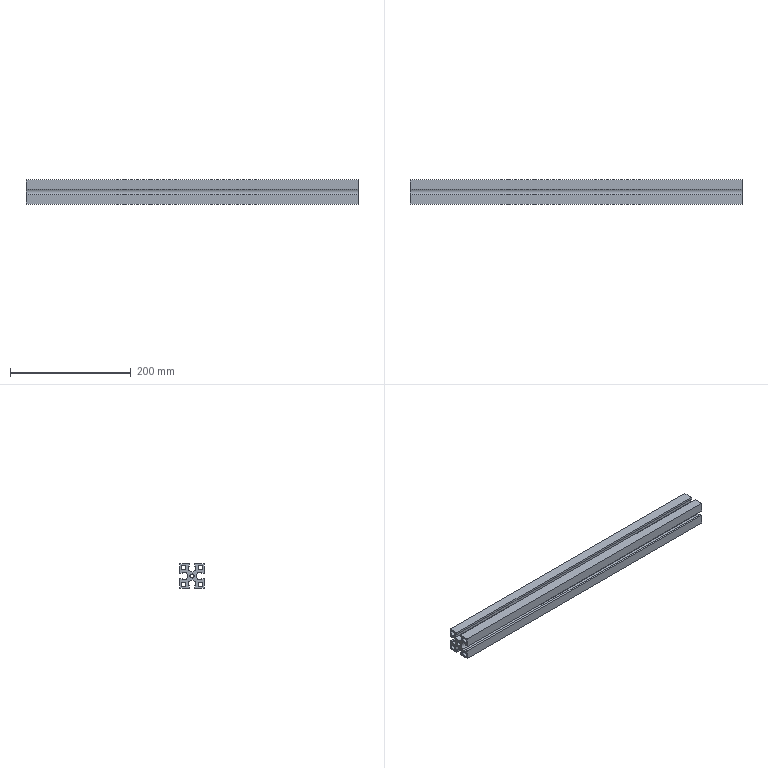Part | NX | 1 solid | 43 faces | box 550 x 40 x 40 mm | volume 437741 mm3 | plane 34 | cylinder 9 | commonest cylinder face diameters 8 x4 20 x4 6.8 x1
STEP:
#1=CARTESIAN_POINT('',(0.,20.,4.25));
#2=VERTEX_POINT('',#1);
#3=CARTESIAN_POINT('',(0.,20.,20.));
#4=VERTEX_POINT('',#3);
#5=CARTESIAN_POINT('',(0.,20.,4.25));
#6=DIRECTION('',(0.,0.,1.));
#7=VECTOR('',#6,1000.);
#8=LINE('',#5,#7);
#9=EDGE_CURVE('',#2,#4,#8,.T.);
#10=ORIENTED_EDGE('',*,*,#9,.T.);
#11=CARTESIAN_POINT('',(550.,20.,20.));
#12=VERTEX_POINT('',#11);
#13=CARTESIAN_POINT('',(550.,20.,20.));
#14=DIRECTION('',(-1.,0.,0.));
#15=VECTOR('',#14,1000.);
#16=LINE('',#13,#15);
#17=EDGE_CURVE('',#12,#4,#16,.T.);
#18=ORIENTED_EDGE('',*,*,#17,.F.);
#19=CARTESIAN_POINT('',(550.,20.,4.25));
#20=VERTEX_POINT('',#19);
#21=CARTESIAN_POINT('',(550.,20.,4.25));
#22=DIRECTION('',(0.,0.,1.));
#23=VECTOR('',#22,1000.);
#24=LINE('',#21,#23);
#25=EDGE_CURVE('',#20,#12,#24,.T.);
#26=ORIENTED_EDGE('',*,*,#25,.F.);
#27=CARTESIAN_POINT('',(550.,20.,4.25));
#28=DIRECTION('',(-1.,0.,0.));
#29=VECTOR('',#28,1000.);
#30=LINE('',#27,#29);
#31=EDGE_CURVE('',#20,#2,#30,.T.);
#32=ORIENTED_EDGE('',*,*,#31,.T.);
#33=EDGE_LOOP('',(#10,#18,#26,#32));
#34=FACE_BOUND('',#33,.T.);
#35=CARTESIAN_POINT('',(550.,20.,4.25));
#36=DIRECTION('',(0.,-1.,0.));
#37=DIRECTION('',(0.,0.,-1.));
#38=AXIS2_PLACEMENT_3D('',#35,#36,#37);
#39=PLANE('',#38);
#40=ADVANCED_FACE('',(#34),#39,.F.);
#41=CARTESIAN_POINT('',(0.,4.25,20.));
#42=VERTEX_POINT('',#41);
#43=CARTESIAN_POINT('',(0.,20.,20.));
#44=DIRECTION('',(0.,-1.,0.));
#45=VECTOR('',#44,1000.);
#46=LINE('',#43,#45);
#47=EDGE_CURVE('',#4,#42,#46,.T.);
#48=ORIENTED_EDGE('',*,*,#47,.T.);
#49=CARTESIAN_POINT('',(550.,4.25,20.));
#50=VERTEX_POINT('',#49);
#51=CARTESIAN_POINT('',(550.,4.25,20.));
#52=DIRECTION('',(-1.,0.,0.));
#53=VECTOR('',#52,1000.);
#54=LINE('',#51,#53);
#55=EDGE_CURVE('',#50,#42,#54,.T.);
#56=ORIENTED_EDGE('',*,*,#55,.F.);
#57=CARTESIAN_POINT('',(550.,20.,20.));
#58=DIRECTION('',(0.,-1.,0.));
#59=VECTOR('',#58,1000.);
#60=LINE('',#57,#59);
#61=EDGE_CURVE('',#12,#50,#60,.T.);
#62=ORIENTED_EDGE('',*,*,#61,.F.);
#63=ORIENTED_EDGE('',*,*,#17,.T.);
#64=EDGE_LOOP('',(#48,#56,#62,#63));
#65=FACE_BOUND('',#64,.T.);
#66=CARTESIAN_POINT('',(550.,20.,20.));
#67=DIRECTION('',(0.,0.,-1.));
#68=DIRECTION('',(0.,1.,0.));
#69=AXIS2_PLACEMENT_3D('',#66,#67,#68);
#70=PLANE('',#69);
#71=ADVANCED_FACE('',(#65),#70,.F.);
#72=CARTESIAN_POINT('',(0.,4.25,16.5));
#73=VERTEX_POINT('',#72);
#74=CARTESIAN_POINT('',(0.,4.25,20.));
#75=DIRECTION('',(0.,0.,-1.));
#76=VECTOR('',#75,1000.);
#77=LINE('',#74,#76);
#78=EDGE_CURVE('',#42,#73,#77,.T.);
#79=ORIENTED_EDGE('',*,*,#78,.T.);
#80=CARTESIAN_POINT('',(550.,4.25,16.5));
#81=VERTEX_POINT('',#80);
#82=CARTESIAN_POINT('',(550.,4.25,16.5));
#83=DIRECTION('',(-1.,0.,0.));
#84=VECTOR('',#83,1000.);
#85=LINE('',#82,#84);
#86=EDGE_CURVE('',#81,#73,#85,.T.);
#87=ORIENTED_EDGE('',*,*,#86,.F.);
#88=CARTESIAN_POINT('',(550.,4.25,20.));
#89=DIRECTION('',(0.,0.,-1.));
#90=VECTOR('',#89,1000.);
#91=LINE('',#88,#90);
#92=EDGE_CURVE('',#50,#81,#91,.T.);
#93=ORIENTED_EDGE('',*,*,#92,.F.);
#94=ORIENTED_EDGE('',*,*,#55,.T.);
#95=EDGE_LOOP('',(#79,#87,#93,#94));
#96=FACE_BOUND('',#95,.T.);
#97=CARTESIAN_POINT('',(550.,4.25,20.));
#98=DIRECTION('',(0.,1.,0.));
#99=DIRECTION('',(0.,0.,1.));
#100=AXIS2_PLACEMENT_3D('',#97,#98,#99);
#101=PLANE('',#100);
#102=ADVANCED_FACE('',(#96),#101,.F.);
#103=CARTESIAN_POINT('',(0.,6.573,16.5));
#104=VERTEX_POINT('',#103);
#105=CARTESIAN_POINT('',(0.,4.25,16.5));
#106=DIRECTION('',(0.,1.,0.));
#107=VECTOR('',#106,1000.);
#108=LINE('',#105,#107);
#109=EDGE_CURVE('',#73,#104,#108,.T.);
#110=ORIENTED_EDGE('',*,*,#109,.T.);
#111=CARTESIAN_POINT('',(550.,6.573,16.5));
#112=VERTEX_POINT('',#111);
#113=CARTESIAN_POINT('',(550.,6.573,16.5));
#114=DIRECTION('',(-1.,0.,0.));
#115=VECTOR('',#114,1000.);
#116=LINE('',#113,#115);
#117=EDGE_CURVE('',#112,#104,#116,.T.);
#118=ORIENTED_EDGE('',*,*,#117,.F.);
#119=CARTESIAN_POINT('',(550.,4.25,16.5));
#120=DIRECTION('',(0.,1.,0.));
#121=VECTOR('',#120,1000.);
#122=LINE('',#119,#121);
#123=EDGE_CURVE('',#81,#112,#122,.T.);
#124=ORIENTED_EDGE('',*,*,#123,.F.);
#125=ORIENTED_EDGE('',*,*,#86,.T.);
#126=EDGE_LOOP('',(#110,#118,#124,#125));
#127=FACE_BOUND('',#126,.T.);
#128=CARTESIAN_POINT('',(550.,4.25,16.5));
#129=DIRECTION('',(0.,0.,1.));
#130=DIRECTION('',(1.,0.,0.));
#131=AXIS2_PLACEMENT_3D('',#128,#129,#130);
#132=PLANE('',#131);
#133=ADVANCED_FACE('',(#127),#132,.F.);
#134=CARTESIAN_POINT('',(0.,6.573,9.673));
#135=VERTEX_POINT('',#134);
#136=CARTESIAN_POINT('',(0.,6.573,16.5));
#137=DIRECTION('',(0.,0.,-1.));
#138=VECTOR('',#137,1000.);
#139=LINE('',#136,#138);
#140=EDGE_CURVE('',#104,#135,#139,.T.);
#141=ORIENTED_EDGE('',*,*,#140,.T.);
#142=CARTESIAN_POINT('',(550.,6.573,9.673));
#143=VERTEX_POINT('',#142);
#144=CARTESIAN_POINT('',(550.,6.573,9.673));
#145=DIRECTION('',(-1.,0.,0.));
#146=VECTOR('',#145,1000.);
#147=LINE('',#144,#146);
#148=EDGE_CURVE('',#143,#135,#147,.T.);
#149=ORIENTED_EDGE('',*,*,#148,.F.);
#150=CARTESIAN_POINT('',(550.,6.573,16.5));
#151=DIRECTION('',(0.,0.,-1.));
#152=VECTOR('',#151,1000.);
#153=LINE('',#150,#152);
#154=EDGE_CURVE('',#112,#143,#153,.T.);
#155=ORIENTED_EDGE('',*,*,#154,.F.);
#156=ORIENTED_EDGE('',*,*,#117,.T.);
#157=EDGE_LOOP('',(#141,#149,#155,#156));
#158=FACE_BOUND('',#157,.T.);
#159=CARTESIAN_POINT('',(550.,6.573,16.5));
#160=DIRECTION('',(0.,1.,0.));
#161=DIRECTION('',(0.,0.,1.));
#162=AXIS2_PLACEMENT_3D('',#159,#160,#161);
#163=PLANE('',#162);
#164=ADVANCED_FACE('',(#158),#163,.F.);
#165=CARTESIAN_POINT('',(0.,-6.573,9.673));
#166=VERTEX_POINT('',#165);
#167=CARTESIAN_POINT('',(0.,0.,17.209));
#168=DIRECTION('',(-1.,0.,0.));
#169=DIRECTION('',(0.,0.,1.));
#170=AXIS2_PLACEMENT_3D('',#167,#168,#169);
#171=CIRCLE('',#170,10.);
#172=EDGE_CURVE('',#135,#166,#171,.T.);
#173=ORIENTED_EDGE('',*,*,#172,.T.);
#174=CARTESIAN_POINT('',(550.,-6.573,9.673));
#175=VERTEX_POINT('',#174);
#176=CARTESIAN_POINT('',(550.,-6.573,9.673));
#177=DIRECTION('',(-1.,0.,0.));
#178=VECTOR('',#177,1000.);
#179=LINE('',#176,#178);
#180=EDGE_CURVE('',#175,#166,#179,.T.);
#181=ORIENTED_EDGE('',*,*,#180,.F.);
#182=CARTESIAN_POINT('',(550.,0.,17.209));
#183=DIRECTION('',(-1.,0.,0.));
#184=DIRECTION('',(0.,0.,1.));
#185=AXIS2_PLACEMENT_3D('',#182,#183,#184);
#186=CIRCLE('',#185,10.);
#187=EDGE_CURVE('',#143,#175,#186,.T.);
#188=ORIENTED_EDGE('',*,*,#187,.F.);
#189=ORIENTED_EDGE('',*,*,#148,.T.);
#190=EDGE_LOOP('',(#173,#181,#188,#189));
#191=FACE_BOUND('',#190,.T.);
#192=CARTESIAN_POINT('',(550.,0.,17.209));
#193=DIRECTION('',(-1.,0.,0.));
#194=DIRECTION('',(0.,0.,1.));
#195=AXIS2_PLACEMENT_3D('',#192,#193,#194);
#196=CYLINDRICAL_SURFACE('',#195,10.);
#197=ADVANCED_FACE('',(#191),#196,.F.);
#198=CARTESIAN_POINT('',(0.,-6.573,16.5));
#199=VERTEX_POINT('',#198);
#200=CARTESIAN_POINT('',(0.,-6.573,9.673));
#201=DIRECTION('',(0.,0.,1.));
#202=VECTOR('',#201,1000.);
#203=LINE('',#200,#202);
#204=EDGE_CURVE('',#166,#199,#203,.T.);
#205=ORIENTED_EDGE('',*,*,#204,.T.);
#206=CARTESIAN_POINT('',(550.,-6.573,16.5));
#207=VERTEX_POINT('',#206);
#208=CARTESIAN_POINT('',(550.,-6.573,16.5));
#209=DIRECTION('',(-1.,0.,0.));
#210=VECTOR('',#209,1000.);
#211=LINE('',#208,#210);
#212=EDGE_CURVE('',#207,#199,#211,.T.);
#213=ORIENTED_EDGE('',*,*,#212,.F.);
#214=CARTESIAN_POINT('',(550.,-6.573,9.673));
#215=DIRECTION('',(0.,0.,1.));
#216=VECTOR('',#215,1000.);
#217=LINE('',#214,#216);
#218=EDGE_CURVE('',#175,#207,#217,.T.);
#219=ORIENTED_EDGE('',*,*,#218,.F.);
#220=ORIENTED_EDGE('',*,*,#180,.T.);
#221=EDGE_LOOP('',(#205,#213,#219,#220));
#222=FACE_BOUND('',#221,.T.);
#223=CARTESIAN_POINT('',(550.,-6.573,9.673));
#224=DIRECTION('',(0.,-1.,0.));
#225=DIRECTION('',(0.,0.,-1.));
#226=AXIS2_PLACEMENT_3D('',#223,#224,#225);
#227=PLANE('',#226);
#228=ADVANCED_FACE('',(#222),#227,.F.);
#229=CARTESIAN_POINT('',(0.,-4.25,16.5));
#230=VERTEX_POINT('',#229);
#231=CARTESIAN_POINT('',(0.,-6.573,16.5));
#232=DIRECTION('',(0.,1.,0.));
#233=VECTOR('',#232,1000.);
#234=LINE('',#231,#233);
#235=EDGE_CURVE('',#199,#230,#234,.T.);
#236=ORIENTED_EDGE('',*,*,#235,.T.);
#237=CARTESIAN_POINT('',(550.,-4.25,16.5));
#238=VERTEX_POINT('',#237);
#239=CARTESIAN_POINT('',(550.,-4.25,16.5));
#240=DIRECTION('',(-1.,0.,0.));
#241=VECTOR('',#240,1000.);
#242=LINE('',#239,#241);
#243=EDGE_CURVE('',#238,#230,#242,.T.);
#244=ORIENTED_EDGE('',*,*,#243,.F.);
#245=CARTESIAN_POINT('',(550.,-6.573,16.5));
#246=DIRECTION('',(0.,1.,0.));
#247=VECTOR('',#246,1000.);
#248=LINE('',#245,#247);
#249=EDGE_CURVE('',#207,#238,#248,.T.);
#250=ORIENTED_EDGE('',*,*,#249,.F.);
#251=ORIENTED_EDGE('',*,*,#212,.T.);
#252=EDGE_LOOP('',(#236,#244,#250,#251));
#253=FACE_BOUND('',#252,.T.);
#254=CARTESIAN_POINT('',(550.,-6.573,16.5));
#255=DIRECTION('',(0.,0.,1.));
#256=DIRECTION('',(1.,0.,0.));
#257=AXIS2_PLACEMENT_3D('',#254,#255,#256);
#258=PLANE('',#257);
#259=ADVANCED_FACE('',(#253),#258,.F.);
#260=CARTESIAN_POINT('',(0.,-4.25,20.));
#261=VERTEX_POINT('',#260);
#262=CARTESIAN_POINT('',(0.,-4.25,16.5));
#263=DIRECTION('',(0.,0.,1.));
#264=VECTOR('',#263,1000.);
#265=LINE('',#262,#264);
#266=EDGE_CURVE('',#230,#261,#265,.T.);
#267=ORIENTED_EDGE('',*,*,#266,.T.);
#268=CARTESIAN_POINT('',(550.,-4.25,20.));
#269=VERTEX_POINT('',#268);
#270=CARTESIAN_POINT('',(550.,-4.25,20.));
#271=DIRECTION('',(-1.,0.,0.));
#272=VECTOR('',#271,1000.);
#273=LINE('',#270,#272);
#274=EDGE_CURVE('',#269,#261,#273,.T.);
#275=ORIENTED_EDGE('',*,*,#274,.F.);
#276=CARTESIAN_POINT('',(550.,-4.25,16.5));
#277=DIRECTION('',(0.,0.,1.));
#278=VECTOR('',#277,1000.);
#279=LINE('',#276,#278);
#280=EDGE_CURVE('',#238,#269,#279,.T.);
#281=ORIENTED_EDGE('',*,*,#280,.F.);
#282=ORIENTED_EDGE('',*,*,#243,.T.);
#283=EDGE_LOOP('',(#267,#275,#281,#282));
#284=FACE_BOUND('',#283,.T.);
#285=CARTESIAN_POINT('',(550.,-4.25,16.5));
#286=DIRECTION('',(0.,-1.,0.));
#287=DIRECTION('',(0.,0.,-1.));
#288=AXIS2_PLACEMENT_3D('',#285,#286,#287);
#289=PLANE('',#288);
#290=ADVANCED_FACE('',(#284),#289,.F.);
#291=CARTESIAN_POINT('',(0.,-20.,20.));
#292=VERTEX_POINT('',#291);
#293=CARTESIAN_POINT('',(0.,-4.25,20.));
#294=DIRECTION('',(0.,-1.,0.));
#295=VECTOR('',#294,1000.);
#296=LINE('',#293,#295);
#297=EDGE_CURVE('',#261,#292,#296,.T.);
#298=ORIENTED_EDGE('',*,*,#297,.T.);
#299=CARTESIAN_POINT('',(550.,-20.,20.));
#300=VERTEX_POINT('',#299);
#301=CARTESIAN_POINT('',(550.,-20.,20.));
#302=DIRECTION('',(-1.,0.,0.));
#303=VECTOR('',#302,1000.);
#304=LINE('',#301,#303);
#305=EDGE_CURVE('',#300,#292,#304,.T.);
#306=ORIENTED_EDGE('',*,*,#305,.F.);
#307=CARTESIAN_POINT('',(550.,-4.25,20.));
#308=DIRECTION('',(0.,-1.,0.));
#309=VECTOR('',#308,1000.);
#310=LINE('',#307,#309);
#311=EDGE_CURVE('',#269,#300,#310,.T.);
#312=ORIENTED_EDGE('',*,*,#311,.F.);
#313=ORIENTED_EDGE('',*,*,#274,.T.);
#314=EDGE_LOOP('',(#298,#306,#312,#313));
#315=FACE_BOUND('',#314,.T.);
#316=CARTESIAN_POINT('',(550.,-4.25,20.));
#317=DIRECTION('',(0.,0.,-1.));
#318=DIRECTION('',(0.,1.,0.));
#319=AXIS2_PLACEMENT_3D('',#316,#317,#318);
#320=PLANE('',#319);
#321=ADVANCED_FACE('',(#315),#320,.F.);
#322=CARTESIAN_POINT('',(0.,-20.,4.25));
#323=VERTEX_POINT('',#322);
#324=CARTESIAN_POINT('',(0.,-20.,20.));
#325=DIRECTION('',(0.,0.,-1.));
#326=VECTOR('',#325,1000.);
#327=LINE('',#324,#326);
#328=EDGE_CURVE('',#292,#323,#327,.T.);
#329=ORIENTED_EDGE('',*,*,#328,.T.);
#330=CARTESIAN_POINT('',(550.,-20.,4.25));
#331=VERTEX_POINT('',#330);
#332=CARTESIAN_POINT('',(550.,-20.,4.25));
#333=DIRECTION('',(-1.,0.,0.));
#334=VECTOR('',#333,1000.);
#335=LINE('',#332,#334);
#336=EDGE_CURVE('',#331,#323,#335,.T.);
#337=ORIENTED_EDGE('',*,*,#336,.F.);
#338=CARTESIAN_POINT('',(550.,-20.,20.));
#339=DIRECTION('',(0.,0.,-1.));
#340=VECTOR('',#339,1000.);
#341=LINE('',#338,#340);
#342=EDGE_CURVE('',#300,#331,#341,.T.);
#343=ORIENTED_EDGE('',*,*,#342,.F.);
#344=ORIENTED_EDGE('',*,*,#305,.T.);
#345=EDGE_LOOP('',(#329,#337,#343,#344));
#346=FACE_BOUND('',#345,.T.);
#347=CARTESIAN_POINT('',(550.,-20.,20.));
#348=DIRECTION('',(0.,1.,0.));
#349=DIRECTION('',(0.,0.,1.));
#350=AXIS2_PLACEMENT_3D('',#347,#348,#349);
#351=PLANE('',#350);
#352=ADVANCED_FACE('',(#346),#351,.F.);
#353=CARTESIAN_POINT('',(0.,-16.5,4.25));
#354=VERTEX_POINT('',#353);
#355=CARTESIAN_POINT('',(0.,-20.,4.25));
#356=DIRECTION('',(0.,1.,0.));
#357=VECTOR('',#356,1000.);
#358=LINE('',#355,#357);
#359=EDGE_CURVE('',#323,#354,#358,.T.);
#360=ORIENTED_EDGE('',*,*,#359,.T.);
#361=CARTESIAN_POINT('',(550.,-16.5,4.25));
#362=VERTEX_POINT('',#361);
#363=CARTESIAN_POINT('',(550.,-16.5,4.25));
#364=DIRECTION('',(-1.,0.,0.));
#365=VECTOR('',#364,1000.);
#366=LINE('',#363,#365);
#367=EDGE_CURVE('',#362,#354,#366,.T.);
#368=ORIENTED_EDGE('',*,*,#367,.F.);
#369=CARTESIAN_POINT('',(550.,-20.,4.25));
#370=DIRECTION('',(0.,1.,0.));
#371=VECTOR('',#370,1000.);
#372=LINE('',#369,#371);
#373=EDGE_CURVE('',#331,#362,#372,.T.);
#374=ORIENTED_EDGE('',*,*,#373,.F.);
#375=ORIENTED_EDGE('',*,*,#336,.T.);
#376=EDGE_LOOP('',(#360,#368,#374,#375));
#377=FACE_BOUND('',#376,.T.);
#378=CARTESIAN_POINT('',(550.,-20.,4.25));
#379=DIRECTION('',(0.,0.,1.));
#380=DIRECTION('',(0.,-1.,0.));
#381=AXIS2_PLACEMENT_3D('',#378,#379,#380);
#382=PLANE('',#381);
#383=ADVANCED_FACE('',(#377),#382,.F.);
#384=CARTESIAN_POINT('',(0.,-16.5,6.573));
#385=VERTEX_POINT('',#384);
#386=CARTESIAN_POINT('',(0.,-16.5,4.25));
#387=DIRECTION('',(0.,0.,1.));
#388=VECTOR('',#387,1000.);
#389=LINE('',#386,#388);
#390=EDGE_CURVE('',#354,#385,#389,.T.);
#391=ORIENTED_EDGE('',*,*,#390,.T.);
#392=CARTESIAN_POINT('',(550.,-16.5,6.573));
#393=VERTEX_POINT('',#392);
#394=CARTESIAN_POINT('',(550.,-16.5,6.573));
#395=DIRECTION('',(-1.,0.,0.));
#396=VECTOR('',#395,1000.);
#397=LINE('',#394,#396);
#398=EDGE_CURVE('',#393,#385,#397,.T.);
#399=ORIENTED_EDGE('',*,*,#398,.F.);
#400=CARTESIAN_POINT('',(550.,-16.5,4.25));
#401=DIRECTION('',(0.,0.,1.));
#402=VECTOR('',#401,1000.);
#403=LINE('',#400,#402);
#404=EDGE_CURVE('',#362,#393,#403,.T.);
#405=ORIENTED_EDGE('',*,*,#404,.F.);
#406=ORIENTED_EDGE('',*,*,#367,.T.);
#407=EDGE_LOOP('',(#391,#399,#405,#406));
#408=FACE_BOUND('',#407,.T.);
#409=CARTESIAN_POINT('',(550.,-16.5,4.25));
#410=DIRECTION('',(0.,-1.,0.));
#411=DIRECTION('',(0.,0.,-1.));
#412=AXIS2_PLACEMENT_3D('',#409,#410,#411);
#413=PLANE('',#412);
#414=ADVANCED_FACE('',(#408),#413,.F.);
#415=CARTESIAN_POINT('',(0.,-9.673,6.573));
#416=VERTEX_POINT('',#415);
#417=CARTESIAN_POINT('',(0.,-16.5,6.573));
#418=DIRECTION('',(0.,1.,0.));
#419=VECTOR('',#418,1000.);
#420=LINE('',#417,#419);
#421=EDGE_CURVE('',#385,#416,#420,.T.);
#422=ORIENTED_EDGE('',*,*,#421,.T.);
#423=CARTESIAN_POINT('',(550.,-9.673,6.573));
#424=VERTEX_POINT('',#423);
#425=CARTESIAN_POINT('',(550.,-9.673,6.573));
#426=DIRECTION('',(-1.,0.,0.));
#427=VECTOR('',#426,1000.);
#428=LINE('',#425,#427);
#429=EDGE_CURVE('',#424,#416,#428,.T.);
#430=ORIENTED_EDGE('',*,*,#429,.F.);
#431=CARTESIAN_POINT('',(550.,-16.5,6.573));
#432=DIRECTION('',(0.,1.,0.));
#433=VECTOR('',#432,1000.);
#434=LINE('',#431,#433);
#435=EDGE_CURVE('',#393,#424,#434,.T.);
#436=ORIENTED_EDGE('',*,*,#435,.F.);
#437=ORIENTED_EDGE('',*,*,#398,.T.);
#438=EDGE_LOOP('',(#422,#430,#436,#437));
#439=FACE_BOUND('',#438,.T.);
#440=CARTESIAN_POINT('',(550.,-16.5,6.573));
#441=DIRECTION('',(0.,0.,1.));
#442=DIRECTION('',(0.,-1.,0.));
#443=AXIS2_PLACEMENT_3D('',#440,#441,#442);
#444=PLANE('',#443);
#445=ADVANCED_FACE('',(#439),#444,.F.);
#446=CARTESIAN_POINT('',(0.,-9.673,-6.573));
#447=VERTEX_POINT('',#446);
#448=CARTESIAN_POINT('',(0.,-17.209,0.));
#449=DIRECTION('',(-1.,0.,0.));
#450=DIRECTION('',(0.,0.,1.));
#451=AXIS2_PLACEMENT_3D('',#448,#449,#450);
#452=CIRCLE('',#451,10.);
#453=EDGE_CURVE('',#416,#447,#452,.T.);
#454=ORIENTED_EDGE('',*,*,#453,.T.);
#455=CARTESIAN_POINT('',(550.,-9.673,-6.573));
#456=VERTEX_POINT('',#455);
#457=CARTESIAN_POINT('',(550.,-9.673,-6.573));
#458=DIRECTION('',(-1.,0.,0.));
#459=VECTOR('',#458,1000.);
#460=LINE('',#457,#459);
#461=EDGE_CURVE('',#456,#447,#460,.T.);
#462=ORIENTED_EDGE('',*,*,#461,.F.);
#463=CARTESIAN_POINT('',(550.,-17.209,0.));
#464=DIRECTION('',(-1.,0.,0.));
#465=DIRECTION('',(0.,0.,1.));
#466=AXIS2_PLACEMENT_3D('',#463,#464,#465);
#467=CIRCLE('',#466,10.);
#468=EDGE_CURVE('',#424,#456,#467,.T.);
#469=ORIENTED_EDGE('',*,*,#468,.F.);
#470=ORIENTED_EDGE('',*,*,#429,.T.);
#471=EDGE_LOOP('',(#454,#462,#469,#470));
#472=FACE_BOUND('',#471,.T.);
#473=CARTESIAN_POINT('',(550.,-17.209,0.));
#474=DIRECTION('',(-1.,0.,0.));
#475=DIRECTION('',(0.,0.,1.));
#476=AXIS2_PLACEMENT_3D('',#473,#474,#475);
#477=CYLINDRICAL_SURFACE('',#476,10.);
#478=ADVANCED_FACE('',(#472),#477,.F.);
#479=CARTESIAN_POINT('',(0.,-16.5,-6.573));
#480=VERTEX_POINT('',#479);
#481=CARTESIAN_POINT('',(0.,-9.673,-6.573));
#482=DIRECTION('',(0.,-1.,0.));
#483=VECTOR('',#482,1000.);
#484=LINE('',#481,#483);
#485=EDGE_CURVE('',#447,#480,#484,.T.);
#486=ORIENTED_EDGE('',*,*,#485,.T.);
#487=CARTESIAN_POINT('',(550.,-16.5,-6.573));
#488=VERTEX_POINT('',#487);
#489=CARTESIAN_POINT('',(550.,-16.5,-6.573));
#490=DIRECTION('',(-1.,0.,0.));
#491=VECTOR('',#490,1000.);
#492=LINE('',#489,#491);
#493=EDGE_CURVE('',#488,#480,#492,.T.);
#494=ORIENTED_EDGE('',*,*,#493,.F.);
#495=CARTESIAN_POINT('',(550.,-9.673,-6.573));
#496=DIRECTION('',(0.,-1.,0.));
#497=VECTOR('',#496,1000.);
#498=LINE('',#495,#497);
#499=EDGE_CURVE('',#456,#488,#498,.T.);
#500=ORIENTED_EDGE('',*,*,#499,.F.);
#501=ORIENTED_EDGE('',*,*,#461,.T.);
#502=EDGE_LOOP('',(#486,#494,#500,#501));
#503=FACE_BOUND('',#502,.T.);
#504=CARTESIAN_POINT('',(550.,-9.673,-6.573));
#505=DIRECTION('',(0.,0.,-1.));
#506=DIRECTION('',(0.,1.,0.));
#507=AXIS2_PLACEMENT_3D('',#504,#505,#506);
#508=PLANE('',#507);
#509=ADVANCED_FACE('',(#503),#508,.F.);
#510=CARTESIAN_POINT('',(0.,-16.5,-4.25));
#511=VERTEX_POINT('',#510);
#512=CARTESIAN_POINT('',(0.,-16.5,-6.573));
#513=DIRECTION('',(0.,0.,1.));
#514=VECTOR('',#513,1000.);
#515=LINE('',#512,#514);
#516=EDGE_CURVE('',#480,#511,#515,.T.);
#517=ORIENTED_EDGE('',*,*,#516,.T.);
#518=CARTESIAN_POINT('',(550.,-16.5,-4.25));
#519=VERTEX_POINT('',#518);
#520=CARTESIAN_POINT('',(550.,-16.5,-4.25));
#521=DIRECTION('',(-1.,0.,0.));
#522=VECTOR('',#521,1000.);
#523=LINE('',#520,#522);
#524=EDGE_CURVE('',#519,#511,#523,.T.);
#525=ORIENTED_EDGE('',*,*,#524,.F.);
#526=CARTESIAN_POINT('',(550.,-16.5,-6.573));
#527=DIRECTION('',(0.,0.,1.));
#528=VECTOR('',#527,1000.);
#529=LINE('',#526,#528);
#530=EDGE_CURVE('',#488,#519,#529,.T.);
#531=ORIENTED_EDGE('',*,*,#530,.F.);
#532=ORIENTED_EDGE('',*,*,#493,.T.);
#533=EDGE_LOOP('',(#517,#525,#531,#532));
#534=FACE_BOUND('',#533,.T.);
#535=CARTESIAN_POINT('',(550.,-16.5,-6.573));
#536=DIRECTION('',(0.,-1.,0.));
#537=DIRECTION('',(0.,0.,-1.));
#538=AXIS2_PLACEMENT_3D('',#535,#536,#537);
#539=PLANE('',#538);
#540=ADVANCED_FACE('',(#534),#539,.F.);
#541=CARTESIAN_POINT('',(0.,-20.,-4.25));
#542=VERTEX_POINT('',#541);
#543=CARTESIAN_POINT('',(0.,-16.5,-4.25));
#544=DIRECTION('',(0.,-1.,0.));
#545=VECTOR('',#544,1000.);
#546=LINE('',#543,#545);
#547=EDGE_CURVE('',#511,#542,#546,.T.);
#548=ORIENTED_EDGE('',*,*,#547,.T.);
#549=CARTESIAN_POINT('',(550.,-20.,-4.25));
#550=VERTEX_POINT('',#549);
#551=CARTESIAN_POINT('',(550.,-20.,-4.25));
#552=DIRECTION('',(-1.,0.,0.));
#553=VECTOR('',#552,1000.);
#554=LINE('',#551,#553);
#555=EDGE_CURVE('',#550,#542,#554,.T.);
#556=ORIENTED_EDGE('',*,*,#555,.F.);
#557=CARTESIAN_POINT('',(550.,-16.5,-4.25));
#558=DIRECTION('',(0.,-1.,0.));
#559=VECTOR('',#558,1000.);
#560=LINE('',#557,#559);
#561=EDGE_CURVE('',#519,#550,#560,.T.);
#562=ORIENTED_EDGE('',*,*,#561,.F.);
#563=ORIENTED_EDGE('',*,*,#524,.T.);
#564=EDGE_LOOP('',(#548,#556,#562,#563));
#565=FACE_BOUND('',#564,.T.);
#566=CARTESIAN_POINT('',(550.,-16.5,-4.25));
#567=DIRECTION('',(0.,0.,-1.));
#568=DIRECTION('',(0.,1.,0.));
#569=AXIS2_PLACEMENT_3D('',#566,#567,#568);
#570=PLANE('',#569);
#571=ADVANCED_FACE('',(#565),#570,.F.);
#572=CARTESIAN_POINT('',(0.,-20.,-20.));
#573=VERTEX_POINT('',#572);
#574=CARTESIAN_POINT('',(0.,-20.,-4.25));
#575=DIRECTION('',(0.,0.,-1.));
#576=VECTOR('',#575,1000.);
#577=LINE('',#574,#576);
#578=EDGE_CURVE('',#542,#573,#577,.T.);
#579=ORIENTED_EDGE('',*,*,#578,.T.);
#580=CARTESIAN_POINT('',(550.,-20.,-20.));
#581=VERTEX_POINT('',#580);
#582=CARTESIAN_POINT('',(550.,-20.,-20.));
#583=DIRECTION('',(-1.,0.,0.));
#584=VECTOR('',#583,1000.);
#585=LINE('',#582,#584);
#586=EDGE_CURVE('',#581,#573,#585,.T.);
#587=ORIENTED_EDGE('',*,*,#586,.F.);
#588=CARTESIAN_POINT('',(550.,-20.,-4.25));
#589=DIRECTION('',(0.,0.,-1.));
#590=VECTOR('',#589,1000.);
#591=LINE('',#588,#590);
#592=EDGE_CURVE('',#550,#581,#591,.T.);
#593=ORIENTED_EDGE('',*,*,#592,.F.);
#594=ORIENTED_EDGE('',*,*,#555,.T.);
#595=EDGE_LOOP('',(#579,#587,#593,#594));
#596=FACE_BOUND('',#595,.T.);
#597=CARTESIAN_POINT('',(550.,-20.,-4.25));
#598=DIRECTION('',(0.,1.,0.));
#599=DIRECTION('',(0.,0.,1.));
#600=AXIS2_PLACEMENT_3D('',#597,#598,#599);
#601=PLANE('',#600);
#602=ADVANCED_FACE('',(#596),#601,.F.);
#603=CARTESIAN_POINT('',(0.,-4.25,-20.));
#604=VERTEX_POINT('',#603);
#605=CARTESIAN_POINT('',(0.,-20.,-20.));
#606=DIRECTION('',(0.,1.,0.));
#607=VECTOR('',#606,1000.);
#608=LINE('',#605,#607);
#609=EDGE_CURVE('',#573,#604,#608,.T.);
#610=ORIENTED_EDGE('',*,*,#609,.T.);
#611=CARTESIAN_POINT('',(550.,-4.25,-20.));
#612=VERTEX_POINT('',#611);
#613=CARTESIAN_POINT('',(550.,-4.25,-20.));
#614=DIRECTION('',(-1.,0.,0.));
#615=VECTOR('',#614,1000.);
#616=LINE('',#613,#615);
#617=EDGE_CURVE('',#612,#604,#616,.T.);
#618=ORIENTED_EDGE('',*,*,#617,.F.);
#619=CARTESIAN_POINT('',(550.,-20.,-20.));
#620=DIRECTION('',(0.,1.,0.));
#621=VECTOR('',#620,1000.);
#622=LINE('',#619,#621);
#623=EDGE_CURVE('',#581,#612,#622,.T.);
#624=ORIENTED_EDGE('',*,*,#623,.F.);
#625=ORIENTED_EDGE('',*,*,#586,.T.);
#626=EDGE_LOOP('',(#610,#618,#624,#625));
#627=FACE_BOUND('',#626,.T.);
#628=CARTESIAN_POINT('',(550.,-20.,-20.));
#629=DIRECTION('',(0.,0.,1.));
#630=DIRECTION('',(1.,0.,0.));
#631=AXIS2_PLACEMENT_3D('',#628,#629,#630);
#632=PLANE('',#631);
#633=ADVANCED_FACE('',(#627),#632,.F.);
#634=CARTESIAN_POINT('',(0.,-4.25,-16.5));
#635=VERTEX_POINT('',#634);
#636=CARTESIAN_POINT('',(0.,-4.25,-20.));
#637=DIRECTION('',(0.,0.,1.));
#638=VECTOR('',#637,1000.);
#639=LINE('',#636,#638);
#640=EDGE_CURVE('',#604,#635,#639,.T.);
#641=ORIENTED_EDGE('',*,*,#640,.T.);
#642=CARTESIAN_POINT('',(550.,-4.25,-16.5));
#643=VERTEX_POINT('',#642);
#644=CARTESIAN_POINT('',(550.,-4.25,-16.5));
#645=DIRECTION('',(-1.,0.,0.));
#646=VECTOR('',#645,1000.);
#647=LINE('',#644,#646);
#648=EDGE_CURVE('',#643,#635,#647,.T.);
#649=ORIENTED_EDGE('',*,*,#648,.F.);
#650=CARTESIAN_POINT('',(550.,-4.25,-20.));
#651=DIRECTION('',(0.,0.,1.));
#652=VECTOR('',#651,1000.);
#653=LINE('',#650,#652);
#654=EDGE_CURVE('',#612,#643,#653,.T.);
#655=ORIENTED_EDGE('',*,*,#654,.F.);
#656=ORIENTED_EDGE('',*,*,#617,.T.);
#657=EDGE_LOOP('',(#641,#649,#655,#656));
#658=FACE_BOUND('',#657,.T.);
#659=CARTESIAN_POINT('',(550.,-4.25,-20.));
#660=DIRECTION('',(0.,-1.,0.));
#661=DIRECTION('',(0.,0.,-1.));
#662=AXIS2_PLACEMENT_3D('',#659,#660,#661);
#663=PLANE('',#662);
#664=ADVANCED_FACE('',(#658),#663,.F.);
#665=CARTESIAN_POINT('',(0.,-6.573,-16.5));
#666=VERTEX_POINT('',#665);
#667=CARTESIAN_POINT('',(0.,-4.25,-16.5));
#668=DIRECTION('',(0.,-1.,0.));
#669=VECTOR('',#668,1000.);
#670=LINE('',#667,#669);
#671=EDGE_CURVE('',#635,#666,#670,.T.);
#672=ORIENTED_EDGE('',*,*,#671,.T.);
#673=CARTESIAN_POINT('',(550.,-6.573,-16.5));
#674=VERTEX_POINT('',#673);
#675=CARTESIAN_POINT('',(550.,-6.573,-16.5));
#676=DIRECTION('',(-1.,0.,0.));
#677=VECTOR('',#676,1000.);
#678=LINE('',#675,#677);
#679=EDGE_CURVE('',#674,#666,#678,.T.);
#680=ORIENTED_EDGE('',*,*,#679,.F.);
#681=CARTESIAN_POINT('',(550.,-4.25,-16.5));
#682=DIRECTION('',(0.,-1.,0.));
#683=VECTOR('',#682,1000.);
#684=LINE('',#681,#683);
#685=EDGE_CURVE('',#643,#674,#684,.T.);
#686=ORIENTED_EDGE('',*,*,#685,.F.);
#687=ORIENTED_EDGE('',*,*,#648,.T.);
#688=EDGE_LOOP('',(#672,#680,#686,#687));
#689=FACE_BOUND('',#688,.T.);
#690=CARTESIAN_POINT('',(550.,-4.25,-16.5));
#691=DIRECTION('',(0.,0.,-1.));
#692=DIRECTION('',(0.,1.,0.));
#693=AXIS2_PLACEMENT_3D('',#690,#691,#692);
#694=PLANE('',#693);
#695=ADVANCED_FACE('',(#689),#694,.F.);
#696=CARTESIAN_POINT('',(0.,-6.573,-9.673));
#697=VERTEX_POINT('',#696);
#698=CARTESIAN_POINT('',(0.,-6.573,-16.5));
#699=DIRECTION('',(0.,0.,1.));
#700=VECTOR('',#699,1000.);
#701=LINE('',#698,#700);
#702=EDGE_CURVE('',#666,#697,#701,.T.);
#703=ORIENTED_EDGE('',*,*,#702,.T.);
#704=CARTESIAN_POINT('',(550.,-6.573,-9.673));
#705=VERTEX_POINT('',#704);
#706=CARTESIAN_POINT('',(550.,-6.573,-9.673));
#707=DIRECTION('',(-1.,0.,0.));
#708=VECTOR('',#707,1000.);
#709=LINE('',#706,#708);
#710=EDGE_CURVE('',#705,#697,#709,.T.);
#711=ORIENTED_EDGE('',*,*,#710,.F.);
#712=CARTESIAN_POINT('',(550.,-6.573,-16.5));
#713=DIRECTION('',(0.,0.,1.));
#714=VECTOR('',#713,1000.);
#715=LINE('',#712,#714);
#716=EDGE_CURVE('',#674,#705,#715,.T.);
#717=ORIENTED_EDGE('',*,*,#716,.F.);
#718=ORIENTED_EDGE('',*,*,#679,.T.);
#719=EDGE_LOOP('',(#703,#711,#717,#718));
#720=FACE_BOUND('',#719,.T.);
#721=CARTESIAN_POINT('',(550.,-6.573,-16.5));
#722=DIRECTION('',(0.,-1.,0.));
#723=DIRECTION('',(0.,0.,-1.));
#724=AXIS2_PLACEMENT_3D('',#721,#722,#723);
#725=PLANE('',#724);
#726=ADVANCED_FACE('',(#720),#725,.F.);
#727=CARTESIAN_POINT('',(0.,6.573,-9.673));
#728=VERTEX_POINT('',#727);
#729=CARTESIAN_POINT('',(0.,0.,-17.209));
#730=DIRECTION('',(-1.,0.,0.));
#731=DIRECTION('',(0.,0.,1.));
#732=AXIS2_PLACEMENT_3D('',#729,#730,#731);
#733=CIRCLE('',#732,10.);
#734=EDGE_CURVE('',#697,#728,#733,.T.);
#735=ORIENTED_EDGE('',*,*,#734,.T.);
#736=CARTESIAN_POINT('',(550.,6.573,-9.673));
#737=VERTEX_POINT('',#736);
#738=CARTESIAN_POINT('',(550.,6.573,-9.673));
#739=DIRECTION('',(-1.,0.,0.));
#740=VECTOR('',#739,1000.);
#741=LINE('',#738,#740);
#742=EDGE_CURVE('',#737,#728,#741,.T.);
#743=ORIENTED_EDGE('',*,*,#742,.F.);
#744=CARTESIAN_POINT('',(550.,0.,-17.209));
#745=DIRECTION('',(-1.,0.,0.));
#746=DIRECTION('',(0.,0.,1.));
#747=AXIS2_PLACEMENT_3D('',#744,#745,#746);
#748=CIRCLE('',#747,10.);
#749=EDGE_CURVE('',#705,#737,#748,.T.);
#750=ORIENTED_EDGE('',*,*,#749,.F.);
#751=ORIENTED_EDGE('',*,*,#710,.T.);
#752=EDGE_LOOP('',(#735,#743,#750,#751));
#753=FACE_BOUND('',#752,.T.);
#754=CARTESIAN_POINT('',(550.,0.,-17.209));
#755=DIRECTION('',(-1.,0.,0.));
#756=DIRECTION('',(0.,0.,1.));
#757=AXIS2_PLACEMENT_3D('',#754,#755,#756);
#758=CYLINDRICAL_SURFACE('',#757,10.);
#759=ADVANCED_FACE('',(#753),#758,.F.);
#760=CARTESIAN_POINT('',(0.,6.573,-16.5));
#761=VERTEX_POINT('',#760);
#762=CARTESIAN_POINT('',(0.,6.573,-9.673));
#763=DIRECTION('',(0.,0.,-1.));
#764=VECTOR('',#763,1000.);
#765=LINE('',#762,#764);
#766=EDGE_CURVE('',#728,#761,#765,.T.);
#767=ORIENTED_EDGE('',*,*,#766,.T.);
#768=CARTESIAN_POINT('',(550.,6.573,-16.5));
#769=VERTEX_POINT('',#768);
#770=CARTESIAN_POINT('',(550.,6.573,-16.5));
#771=DIRECTION('',(-1.,0.,0.));
#772=VECTOR('',#771,1000.);
#773=LINE('',#770,#772);
#774=EDGE_CURVE('',#769,#761,#773,.T.);
#775=ORIENTED_EDGE('',*,*,#774,.F.);
#776=CARTESIAN_POINT('',(550.,6.573,-9.673));
#777=DIRECTION('',(0.,0.,-1.));
#778=VECTOR('',#777,1000.);
#779=LINE('',#776,#778);
#780=EDGE_CURVE('',#737,#769,#779,.T.);
#781=ORIENTED_EDGE('',*,*,#780,.F.);
#782=ORIENTED_EDGE('',*,*,#742,.T.);
#783=EDGE_LOOP('',(#767,#775,#781,#782));
#784=FACE_BOUND('',#783,.T.);
#785=CARTESIAN_POINT('',(550.,6.573,-9.673));
#786=DIRECTION('',(0.,1.,0.));
#787=DIRECTION('',(0.,0.,1.));
#788=AXIS2_PLACEMENT_3D('',#785,#786,#787);
#789=PLANE('',#788);
#790=ADVANCED_FACE('',(#784),#789,.F.);
#791=CARTESIAN_POINT('',(0.,4.25,-16.5));
#792=VERTEX_POINT('',#791);
#793=CARTESIAN_POINT('',(0.,6.573,-16.5));
#794=DIRECTION('',(0.,-1.,0.));
#795=VECTOR('',#794,1000.);
#796=LINE('',#793,#795);
#797=EDGE_CURVE('',#761,#792,#796,.T.);
#798=ORIENTED_EDGE('',*,*,#797,.T.);
#799=CARTESIAN_POINT('',(550.,4.25,-16.5));
#800=VERTEX_POINT('',#799);
#801=CARTESIAN_POINT('',(550.,4.25,-16.5));
#802=DIRECTION('',(-1.,0.,0.));
#803=VECTOR('',#802,1000.);
#804=LINE('',#801,#803);
#805=EDGE_CURVE('',#800,#792,#804,.T.);
#806=ORIENTED_EDGE('',*,*,#805,.F.);
#807=CARTESIAN_POINT('',(550.,6.573,-16.5));
#808=DIRECTION('',(0.,-1.,0.));
#809=VECTOR('',#808,1000.);
#810=LINE('',#807,#809);
#811=EDGE_CURVE('',#769,#800,#810,.T.);
#812=ORIENTED_EDGE('',*,*,#811,.F.);
#813=ORIENTED_EDGE('',*,*,#774,.T.);
#814=EDGE_LOOP('',(#798,#806,#812,#813));
#815=FACE_BOUND('',#814,.T.);
#816=CARTESIAN_POINT('',(550.,6.573,-16.5));
#817=DIRECTION('',(0.,0.,-1.));
#818=DIRECTION('',(0.,1.,0.));
#819=AXIS2_PLACEMENT_3D('',#816,#817,#818);
#820=PLANE('',#819);
#821=ADVANCED_FACE('',(#815),#820,.F.);
#822=CARTESIAN_POINT('',(0.,4.25,-20.));
#823=VERTEX_POINT('',#822);
#824=CARTESIAN_POINT('',(0.,4.25,-16.5));
#825=DIRECTION('',(0.,0.,-1.));
#826=VECTOR('',#825,1000.);
#827=LINE('',#824,#826);
#828=EDGE_CURVE('',#792,#823,#827,.T.);
#829=ORIENTED_EDGE('',*,*,#828,.T.);
#830=CARTESIAN_POINT('',(550.,4.25,-20.));
#831=VERTEX_POINT('',#830);
#832=CARTESIAN_POINT('',(550.,4.25,-20.));
#833=DIRECTION('',(-1.,0.,0.));
#834=VECTOR('',#833,1000.);
#835=LINE('',#832,#834);
#836=EDGE_CURVE('',#831,#823,#835,.T.);
#837=ORIENTED_EDGE('',*,*,#836,.F.);
#838=CARTESIAN_POINT('',(550.,4.25,-16.5));
#839=DIRECTION('',(0.,0.,-1.));
#840=VECTOR('',#839,1000.);
#841=LINE('',#838,#840);
#842=EDGE_CURVE('',#800,#831,#841,.T.);
#843=ORIENTED_EDGE('',*,*,#842,.F.);
#844=ORIENTED_EDGE('',*,*,#805,.T.);
#845=EDGE_LOOP('',(#829,#837,#843,#844));
#846=FACE_BOUND('',#845,.T.);
#847=CARTESIAN_POINT('',(550.,4.25,-16.5));
#848=DIRECTION('',(0.,1.,0.));
#849=DIRECTION('',(0.,0.,1.));
#850=AXIS2_PLACEMENT_3D('',#847,#848,#849);
#851=PLANE('',#850);
#852=ADVANCED_FACE('',(#846),#851,.F.);
#853=CARTESIAN_POINT('',(0.,20.,-20.));
#854=VERTEX_POINT('',#853);
#855=CARTESIAN_POINT('',(0.,4.25,-20.));
#856=DIRECTION('',(0.,1.,0.));
#857=VECTOR('',#856,1000.);
#858=LINE('',#855,#857);
#859=EDGE_CURVE('',#823,#854,#858,.T.);
#860=ORIENTED_EDGE('',*,*,#859,.T.);
#861=CARTESIAN_POINT('',(550.,20.,-20.));
#862=VERTEX_POINT('',#861);
#863=CARTESIAN_POINT('',(550.,20.,-20.));
#864=DIRECTION('',(-1.,0.,0.));
#865=VECTOR('',#864,1000.);
#866=LINE('',#863,#865);
#867=EDGE_CURVE('',#862,#854,#866,.T.);
#868=ORIENTED_EDGE('',*,*,#867,.F.);
#869=CARTESIAN_POINT('',(550.,4.25,-20.));
#870=DIRECTION('',(0.,1.,0.));
#871=VECTOR('',#870,1000.);
#872=LINE('',#869,#871);
#873=EDGE_CURVE('',#831,#862,#872,.T.);
#874=ORIENTED_EDGE('',*,*,#873,.F.);
#875=ORIENTED_EDGE('',*,*,#836,.T.);
#876=EDGE_LOOP('',(#860,#868,#874,#875));
#877=FACE_BOUND('',#876,.T.);
#878=CARTESIAN_POINT('',(550.,4.25,-20.));
#879=DIRECTION('',(0.,0.,1.));
#880=DIRECTION('',(1.,0.,0.));
#881=AXIS2_PLACEMENT_3D('',#878,#879,#880);
#882=PLANE('',#881);
#883=ADVANCED_FACE('',(#877),#882,.F.);
#884=CARTESIAN_POINT('',(0.,20.,-4.25));
#885=VERTEX_POINT('',#884);
#886=CARTESIAN_POINT('',(0.,20.,-20.));
#887=DIRECTION('',(0.,0.,1.));
#888=VECTOR('',#887,1000.);
#889=LINE('',#886,#888);
#890=EDGE_CURVE('',#854,#885,#889,.T.);
#891=ORIENTED_EDGE('',*,*,#890,.T.);
#892=CARTESIAN_POINT('',(550.,20.,-4.25));
#893=VERTEX_POINT('',#892);
#894=CARTESIAN_POINT('',(550.,20.,-4.25));
#895=DIRECTION('',(-1.,0.,0.));
#896=VECTOR('',#895,1000.);
#897=LINE('',#894,#896);
#898=EDGE_CURVE('',#893,#885,#897,.T.);
#899=ORIENTED_EDGE('',*,*,#898,.F.);
#900=CARTESIAN_POINT('',(550.,20.,-20.));
#901=DIRECTION('',(0.,0.,1.));
#902=VECTOR('',#901,1000.);
#903=LINE('',#900,#902);
#904=EDGE_CURVE('',#862,#893,#903,.T.);
#905=ORIENTED_EDGE('',*,*,#904,.F.);
#906=ORIENTED_EDGE('',*,*,#867,.T.);
#907=EDGE_LOOP('',(#891,#899,#905,#906));
#908=FACE_BOUND('',#907,.T.);
#909=CARTESIAN_POINT('',(550.,20.,-20.));
#910=DIRECTION('',(0.,-1.,0.));
#911=DIRECTION('',(0.,0.,-1.));
#912=AXIS2_PLACEMENT_3D('',#909,#910,#911);
#913=PLANE('',#912);
#914=ADVANCED_FACE('',(#908),#913,.F.);
#915=CARTESIAN_POINT('',(0.,16.5,-4.25));
#916=VERTEX_POINT('',#915);
#917=CARTESIAN_POINT('',(0.,20.,-4.25));
#918=DIRECTION('',(0.,-1.,0.));
#919=VECTOR('',#918,1000.);
#920=LINE('',#917,#919);
#921=EDGE_CURVE('',#885,#916,#920,.T.);
#922=ORIENTED_EDGE('',*,*,#921,.T.);
#923=CARTESIAN_POINT('',(550.,16.5,-4.25));
#924=VERTEX_POINT('',#923);
#925=CARTESIAN_POINT('',(550.,16.5,-4.25));
#926=DIRECTION('',(-1.,0.,0.));
#927=VECTOR('',#926,1000.);
#928=LINE('',#925,#927);
#929=EDGE_CURVE('',#924,#916,#928,.T.);
#930=ORIENTED_EDGE('',*,*,#929,.F.);
#931=CARTESIAN_POINT('',(550.,20.,-4.25));
#932=DIRECTION('',(0.,-1.,0.));
#933=VECTOR('',#932,1000.);
#934=LINE('',#931,#933);
#935=EDGE_CURVE('',#893,#924,#934,.T.);
#936=ORIENTED_EDGE('',*,*,#935,.F.);
#937=ORIENTED_EDGE('',*,*,#898,.T.);
#938=EDGE_LOOP('',(#922,#930,#936,#937));
#939=FACE_BOUND('',#938,.T.);
#940=CARTESIAN_POINT('',(550.,20.,-4.25));
#941=DIRECTION('',(0.,0.,-1.));
#942=DIRECTION('',(-1.,0.,0.));
#943=AXIS2_PLACEMENT_3D('',#940,#941,#942);
#944=PLANE('',#943);
#945=ADVANCED_FACE('',(#939),#944,.F.);
#946=CARTESIAN_POINT('',(0.,16.5,-6.573));
#947=VERTEX_POINT('',#946);
#948=CARTESIAN_POINT('',(0.,16.5,-4.25));
#949=DIRECTION('',(0.,0.,-1.));
#950=VECTOR('',#949,1000.);
#951=LINE('',#948,#950);
#952=EDGE_CURVE('',#916,#947,#951,.T.);
#953=ORIENTED_EDGE('',*,*,#952,.T.);
#954=CARTESIAN_POINT('',(550.,16.5,-6.573));
#955=VERTEX_POINT('',#954);
#956=CARTESIAN_POINT('',(550.,16.5,-6.573));
#957=DIRECTION('',(-1.,0.,0.));
#958=VECTOR('',#957,1000.);
#959=LINE('',#956,#958);
#960=EDGE_CURVE('',#955,#947,#959,.T.);
#961=ORIENTED_EDGE('',*,*,#960,.F.);
#962=CARTESIAN_POINT('',(550.,16.5,-4.25));
#963=DIRECTION('',(0.,0.,-1.));
#964=VECTOR('',#963,1000.);
#965=LINE('',#962,#964);
#966=EDGE_CURVE('',#924,#955,#965,.T.);
#967=ORIENTED_EDGE('',*,*,#966,.F.);
#968=ORIENTED_EDGE('',*,*,#929,.T.);
#969=EDGE_LOOP('',(#953,#961,#967,#968));
#970=FACE_BOUND('',#969,.T.);
#971=CARTESIAN_POINT('',(550.,16.5,-4.25));
#972=DIRECTION('',(0.,1.,0.));
#973=DIRECTION('',(0.,0.,1.));
#974=AXIS2_PLACEMENT_3D('',#971,#972,#973);
#975=PLANE('',#974);
#976=ADVANCED_FACE('',(#970),#975,.F.);
#977=CARTESIAN_POINT('',(0.,9.673,-6.573));
#978=VERTEX_POINT('',#977);
#979=CARTESIAN_POINT('',(0.,16.5,-6.573));
#980=DIRECTION('',(0.,-1.,0.));
#981=VECTOR('',#980,1000.);
#982=LINE('',#979,#981);
#983=EDGE_CURVE('',#947,#978,#982,.T.);
#984=ORIENTED_EDGE('',*,*,#983,.T.);
#985=CARTESIAN_POINT('',(550.,9.673,-6.573));
#986=VERTEX_POINT('',#985);
#987=CARTESIAN_POINT('',(550.,9.673,-6.573));
#988=DIRECTION('',(-1.,0.,0.));
#989=VECTOR('',#988,1000.);
#990=LINE('',#987,#989);
#991=EDGE_CURVE('',#986,#978,#990,.T.);
#992=ORIENTED_EDGE('',*,*,#991,.F.);
#993=CARTESIAN_POINT('',(550.,16.5,-6.573));
#994=DIRECTION('',(0.,-1.,0.));
#995=VECTOR('',#994,1000.);
#996=LINE('',#993,#995);
#997=EDGE_CURVE('',#955,#986,#996,.T.);
#998=ORIENTED_EDGE('',*,*,#997,.F.);
#999=ORIENTED_EDGE('',*,*,#960,.T.);
#1000=EDGE_LOOP('',(#984,#992,#998,#999));
#1001=FACE_BOUND('',#1000,.T.);
#1002=CARTESIAN_POINT('',(550.,16.5,-6.573));
#1003=DIRECTION('',(0.,0.,-1.));
#1004=DIRECTION('',(-1.,0.,0.));
#1005=AXIS2_PLACEMENT_3D('',#1002,#1003,#1004);
#1006=PLANE('',#1005);
#1007=ADVANCED_FACE('',(#1001),#1006,.F.);
#1008=CARTESIAN_POINT('',(0.,9.673,6.573));
#1009=VERTEX_POINT('',#1008);
#1010=CARTESIAN_POINT('',(0.,17.209,0.));
#1011=DIRECTION('',(-1.,0.,0.));
#1012=DIRECTION('',(0.,0.,1.));
#1013=AXIS2_PLACEMENT_3D('',#1010,#1011,#1012);
#1014=CIRCLE('',#1013,10.);
#1015=EDGE_CURVE('',#978,#1009,#1014,.T.);
#1016=ORIENTED_EDGE('',*,*,#1015,.T.);
#1017=CARTESIAN_POINT('',(550.,9.673,6.573));
#1018=VERTEX_POINT('',#1017);
#1019=CARTESIAN_POINT('',(550.,9.673,6.573));
#1020=DIRECTION('',(-1.,0.,0.));
#1021=VECTOR('',#1020,1000.);
#1022=LINE('',#1019,#1021);
#1023=EDGE_CURVE('',#1018,#1009,#1022,.T.);
#1024=ORIENTED_EDGE('',*,*,#1023,.F.);
#1025=CARTESIAN_POINT('',(550.,17.209,0.));
#1026=DIRECTION('',(-1.,0.,0.));
#1027=DIRECTION('',(0.,0.,1.));
#1028=AXIS2_PLACEMENT_3D('',#1025,#1026,#1027);
#1029=CIRCLE('',#1028,10.);
#1030=EDGE_CURVE('',#986,#1018,#1029,.T.);
#1031=ORIENTED_EDGE('',*,*,#1030,.F.);
#1032=ORIENTED_EDGE('',*,*,#991,.T.);
#1033=EDGE_LOOP('',(#1016,#1024,#1031,#1032));
#1034=FACE_BOUND('',#1033,.T.);
#1035=CARTESIAN_POINT('',(550.,17.209,0.));
#1036=DIRECTION('',(-1.,0.,0.));
#1037=DIRECTION('',(0.,0.,1.));
#1038=AXIS2_PLACEMENT_3D('',#1035,#1036,#1037);
#1039=CYLINDRICAL_SURFACE('',#1038,10.);
#1040=ADVANCED_FACE('',(#1034),#1039,.F.);
#1041=CARTESIAN_POINT('',(0.,16.5,6.573));
#1042=VERTEX_POINT('',#1041);
#1043=CARTESIAN_POINT('',(0.,9.673,6.573));
#1044=DIRECTION('',(0.,1.,0.));
#1045=VECTOR('',#1044,1000.);
#1046=LINE('',#1043,#1045);
#1047=EDGE_CURVE('',#1009,#1042,#1046,.T.);
#1048=ORIENTED_EDGE('',*,*,#1047,.T.);
#1049=CARTESIAN_POINT('',(550.,16.5,6.573));
#1050=VERTEX_POINT('',#1049);
#1051=CARTESIAN_POINT('',(550.,16.5,6.573));
#1052=DIRECTION('',(-1.,0.,0.));
#1053=VECTOR('',#1052,1000.);
#1054=LINE('',#1051,#1053);
#1055=EDGE_CURVE('',#1050,#1042,#1054,.T.);
#1056=ORIENTED_EDGE('',*,*,#1055,.F.);
#1057=CARTESIAN_POINT('',(550.,9.673,6.573));
#1058=DIRECTION('',(0.,1.,0.));
#1059=VECTOR('',#1058,1000.);
#1060=LINE('',#1057,#1059);
#1061=EDGE_CURVE('',#1018,#1050,#1060,.T.);
#1062=ORIENTED_EDGE('',*,*,#1061,.F.);
#1063=ORIENTED_EDGE('',*,*,#1023,.T.);
#1064=EDGE_LOOP('',(#1048,#1056,#1062,#1063));
#1065=FACE_BOUND('',#1064,.T.);
#1066=CARTESIAN_POINT('',(550.,9.673,6.573));
#1067=DIRECTION('',(0.,0.,1.));
#1068=DIRECTION('',(1.,0.,0.));
#1069=AXIS2_PLACEMENT_3D('',#1066,#1067,#1068);
#1070=PLANE('',#1069);
#1071=ADVANCED_FACE('',(#1065),#1070,.F.);
#1072=CARTESIAN_POINT('',(0.,16.5,4.25));
#1073=VERTEX_POINT('',#1072);
#1074=CARTESIAN_POINT('',(0.,16.5,6.573));
#1075=DIRECTION('',(0.,0.,-1.));
#1076=VECTOR('',#1075,1000.);
#1077=LINE('',#1074,#1076);
#1078=EDGE_CURVE('',#1042,#1073,#1077,.T.);
#1079=ORIENTED_EDGE('',*,*,#1078,.T.);
#1080=CARTESIAN_POINT('',(550.,16.5,4.25));
#1081=VERTEX_POINT('',#1080);
#1082=CARTESIAN_POINT('',(550.,16.5,4.25));
#1083=DIRECTION('',(-1.,0.,0.));
#1084=VECTOR('',#1083,1000.);
#1085=LINE('',#1082,#1084);
#1086=EDGE_CURVE('',#1081,#1073,#1085,.T.);
#1087=ORIENTED_EDGE('',*,*,#1086,.F.);
#1088=CARTESIAN_POINT('',(550.,16.5,6.573));
#1089=DIRECTION('',(0.,0.,-1.));
#1090=VECTOR('',#1089,1000.);
#1091=LINE('',#1088,#1090);
#1092=EDGE_CURVE('',#1050,#1081,#1091,.T.);
#1093=ORIENTED_EDGE('',*,*,#1092,.F.);
#1094=ORIENTED_EDGE('',*,*,#1055,.T.);
#1095=EDGE_LOOP('',(#1079,#1087,#1093,#1094));
#1096=FACE_BOUND('',#1095,.T.);
#1097=CARTESIAN_POINT('',(550.,16.5,6.573));
#1098=DIRECTION('',(0.,1.,0.));
#1099=DIRECTION('',(0.,0.,1.));
#1100=AXIS2_PLACEMENT_3D('',#1097,#1098,#1099);
#1101=PLANE('',#1100);
#1102=ADVANCED_FACE('',(#1096),#1101,.F.);
#1103=CARTESIAN_POINT('',(550.,14.,-10.));
#1104=VERTEX_POINT('',#1103);
#1105=CARTESIAN_POINT('',(550.,14.,-14.));
#1106=DIRECTION('',(1.,0.,0.));
#1107=DIRECTION('',(0.,0.,1.));
#1108=AXIS2_PLACEMENT_3D('',#1105,#1106,#1107);
#1109=CIRCLE('',#1108,4.);
#1110=EDGE_CURVE('',#1104,#1104,#1109,.T.);
#1111=ORIENTED_EDGE('',*,*,#1110,.T.);
#1112=EDGE_LOOP('',(#1111));
#1113=FACE_BOUND('',#1112,.T.);
#1114=CARTESIAN_POINT('',(0.,14.,-10.));
#1115=VERTEX_POINT('',#1114);
#1116=CARTESIAN_POINT('',(0.,14.,-14.));
#1117=DIRECTION('',(1.,0.,0.));
#1118=DIRECTION('',(0.,0.,1.));
#1119=AXIS2_PLACEMENT_3D('',#1116,#1117,#1118);
#1120=CIRCLE('',#1119,4.);
#1121=EDGE_CURVE('',#1115,#1115,#1120,.T.);
#1122=ORIENTED_EDGE('',*,*,#1121,.F.);
#1123=EDGE_LOOP('',(#1122));
#1124=FACE_BOUND('',#1123,.T.);
#1125=CARTESIAN_POINT('',(550.,14.,-14.));
#1126=DIRECTION('',(-1.,0.,0.));
#1127=DIRECTION('',(0.,0.,1.));
#1128=AXIS2_PLACEMENT_3D('',#1125,#1126,#1127);
#1129=CYLINDRICAL_SURFACE('',#1128,4.);
#1130=ADVANCED_FACE('',(#1113,#1124),#1129,.F.);
#1131=CARTESIAN_POINT('',(550.,-14.,18.));
#1132=VERTEX_POINT('',#1131);
#1133=CARTESIAN_POINT('',(550.,-14.,14.));
#1134=DIRECTION('',(1.,0.,0.));
#1135=DIRECTION('',(0.,0.,1.));
#1136=AXIS2_PLACEMENT_3D('',#1133,#1134,#1135);
#1137=CIRCLE('',#1136,4.);
#1138=EDGE_CURVE('',#1132,#1132,#1137,.T.);
#1139=ORIENTED_EDGE('',*,*,#1138,.T.);
#1140=EDGE_LOOP('',(#1139));
#1141=FACE_BOUND('',#1140,.T.);
#1142=CARTESIAN_POINT('',(0.,-14.,18.));
#1143=VERTEX_POINT('',#1142);
#1144=CARTESIAN_POINT('',(0.,-14.,14.));
#1145=DIRECTION('',(1.,0.,0.));
#1146=DIRECTION('',(0.,0.,1.));
#1147=AXIS2_PLACEMENT_3D('',#1144,#1145,#1146);
#1148=CIRCLE('',#1147,4.);
#1149=EDGE_CURVE('',#1143,#1143,#1148,.T.);
#1150=ORIENTED_EDGE('',*,*,#1149,.F.);
#1151=EDGE_LOOP('',(#1150));
#1152=FACE_BOUND('',#1151,.T.);
#1153=CARTESIAN_POINT('',(550.,-14.,14.));
#1154=DIRECTION('',(-1.,0.,0.));
#1155=DIRECTION('',(0.,0.,1.));
#1156=AXIS2_PLACEMENT_3D('',#1153,#1154,#1155);
#1157=CYLINDRICAL_SURFACE('',#1156,4.);
#1158=ADVANCED_FACE('',(#1141,#1152),#1157,.F.);
#1159=CARTESIAN_POINT('',(0.,16.5,4.25));
#1160=DIRECTION('',(0.,1.,0.));
#1161=VECTOR('',#1160,1000.);
#1162=LINE('',#1159,#1161);
#1163=EDGE_CURVE('',#1073,#2,#1162,.T.);
#1164=ORIENTED_EDGE('',*,*,#1163,.T.);
#1165=ORIENTED_EDGE('',*,*,#31,.F.);
#1166=CARTESIAN_POINT('',(550.,16.5,4.25));
#1167=DIRECTION('',(0.,1.,0.));
#1168=VECTOR('',#1167,1000.);
#1169=LINE('',#1166,#1168);
#1170=EDGE_CURVE('',#1081,#20,#1169,.T.);
#1171=ORIENTED_EDGE('',*,*,#1170,.F.);
#1172=ORIENTED_EDGE('',*,*,#1086,.T.);
#1173=EDGE_LOOP('',(#1164,#1165,#1171,#1172));
#1174=FACE_BOUND('',#1173,.T.);
#1175=CARTESIAN_POINT('',(550.,16.5,4.25));
#1176=DIRECTION('',(0.,0.,1.));
#1177=DIRECTION('',(1.,0.,0.));
#1178=AXIS2_PLACEMENT_3D('',#1175,#1176,#1177);
#1179=PLANE('',#1178);
#1180=ADVANCED_FACE('',(#1174),#1179,.F.);
#1181=CARTESIAN_POINT('',(550.,14.,18.));
#1182=VERTEX_POINT('',#1181);
#1183=CARTESIAN_POINT('',(550.,14.,14.));
#1184=DIRECTION('',(1.,0.,0.));
#1185=DIRECTION('',(0.,0.,1.));
#1186=AXIS2_PLACEMENT_3D('',#1183,#1184,#1185);
#1187=CIRCLE('',#1186,4.);
#1188=EDGE_CURVE('',#1182,#1182,#1187,.T.);
#1189=ORIENTED_EDGE('',*,*,#1188,.T.);
#1190=EDGE_LOOP('',(#1189));
#1191=FACE_BOUND('',#1190,.T.);
#1192=CARTESIAN_POINT('',(0.,14.,18.));
#1193=VERTEX_POINT('',#1192);
#1194=CARTESIAN_POINT('',(0.,14.,14.));
#1195=DIRECTION('',(1.,0.,0.));
#1196=DIRECTION('',(0.,0.,1.));
#1197=AXIS2_PLACEMENT_3D('',#1194,#1195,#1196);
#1198=CIRCLE('',#1197,4.);
#1199=EDGE_CURVE('',#1193,#1193,#1198,.T.);
#1200=ORIENTED_EDGE('',*,*,#1199,.F.);
#1201=EDGE_LOOP('',(#1200));
#1202=FACE_BOUND('',#1201,.T.);
#1203=CARTESIAN_POINT('',(550.,14.,14.));
#1204=DIRECTION('',(-1.,0.,0.));
#1205=DIRECTION('',(0.,0.,1.));
#1206=AXIS2_PLACEMENT_3D('',#1203,#1204,#1205);
#1207=CYLINDRICAL_SURFACE('',#1206,4.);
#1208=ADVANCED_FACE('',(#1191,#1202),#1207,.F.);
#1209=CARTESIAN_POINT('',(550.,-14.,-10.));
#1210=VERTEX_POINT('',#1209);
#1211=CARTESIAN_POINT('',(550.,-14.,-14.));
#1212=DIRECTION('',(1.,0.,0.));
#1213=DIRECTION('',(0.,0.,1.));
#1214=AXIS2_PLACEMENT_3D('',#1211,#1212,#1213);
#1215=CIRCLE('',#1214,4.);
#1216=EDGE_CURVE('',#1210,#1210,#1215,.T.);
#1217=ORIENTED_EDGE('',*,*,#1216,.T.);
#1218=EDGE_LOOP('',(#1217));
#1219=FACE_BOUND('',#1218,.T.);
#1220=CARTESIAN_POINT('',(0.,-14.,-10.));
#1221=VERTEX_POINT('',#1220);
#1222=CARTESIAN_POINT('',(0.,-14.,-14.));
#1223=DIRECTION('',(1.,0.,0.));
#1224=DIRECTION('',(0.,0.,1.));
#1225=AXIS2_PLACEMENT_3D('',#1222,#1223,#1224);
#1226=CIRCLE('',#1225,4.);
#1227=EDGE_CURVE('',#1221,#1221,#1226,.T.);
#1228=ORIENTED_EDGE('',*,*,#1227,.F.);
#1229=EDGE_LOOP('',(#1228));
#1230=FACE_BOUND('',#1229,.T.);
#1231=CARTESIAN_POINT('',(550.,-14.,-14.));
#1232=DIRECTION('',(-1.,0.,0.));
#1233=DIRECTION('',(0.,0.,1.));
#1234=AXIS2_PLACEMENT_3D('',#1231,#1232,#1233);
#1235=CYLINDRICAL_SURFACE('',#1234,4.);
#1236=ADVANCED_FACE('',(#1219,#1230),#1235,.F.);
#1237=CARTESIAN_POINT('',(550.,0.,3.4));
#1238=VERTEX_POINT('',#1237);
#1239=CARTESIAN_POINT('',(550.,0.,0.));
#1240=DIRECTION('',(1.,0.,0.));
#1241=DIRECTION('',(0.,0.,1.));
#1242=AXIS2_PLACEMENT_3D('',#1239,#1240,#1241);
#1243=CIRCLE('',#1242,3.4);
#1244=EDGE_CURVE('',#1238,#1238,#1243,.T.);
#1245=ORIENTED_EDGE('',*,*,#1244,.T.);
#1246=EDGE_LOOP('',(#1245));
#1247=FACE_BOUND('',#1246,.T.);
#1248=CARTESIAN_POINT('',(0.,0.,3.4));
#1249=VERTEX_POINT('',#1248);
#1250=CARTESIAN_POINT('',(0.,0.,0.));
#1251=DIRECTION('',(1.,0.,0.));
#1252=DIRECTION('',(0.,0.,1.));
#1253=AXIS2_PLACEMENT_3D('',#1250,#1251,#1252);
#1254=CIRCLE('',#1253,3.4);
#1255=EDGE_CURVE('',#1249,#1249,#1254,.T.);
#1256=ORIENTED_EDGE('',*,*,#1255,.F.);
#1257=EDGE_LOOP('',(#1256));
#1258=FACE_BOUND('',#1257,.T.);
#1259=CARTESIAN_POINT('',(550.,0.,0.));
#1260=DIRECTION('',(-1.,0.,0.));
#1261=DIRECTION('',(0.,0.,1.));
#1262=AXIS2_PLACEMENT_3D('',#1259,#1260,#1261);
#1263=CYLINDRICAL_SURFACE('',#1262,3.4);
#1264=ADVANCED_FACE('',(#1247,#1258),#1263,.F.);
#1265=ORIENTED_EDGE('',*,*,#1216,.F.);
#1266=EDGE_LOOP('',(#1265));
#1267=FACE_BOUND('',#1266,.T.);
#1268=ORIENTED_EDGE('',*,*,#1188,.F.);
#1269=EDGE_LOOP('',(#1268));
#1270=FACE_BOUND('',#1269,.T.);
#1271=ORIENTED_EDGE('',*,*,#25,.T.);
#1272=ORIENTED_EDGE('',*,*,#61,.T.);
#1273=ORIENTED_EDGE('',*,*,#92,.T.);
#1274=ORIENTED_EDGE('',*,*,#123,.T.);
#1275=ORIENTED_EDGE('',*,*,#154,.T.);
#1276=ORIENTED_EDGE('',*,*,#187,.T.);
#1277=ORIENTED_EDGE('',*,*,#218,.T.);
#1278=ORIENTED_EDGE('',*,*,#249,.T.);
#1279=ORIENTED_EDGE('',*,*,#280,.T.);
#1280=ORIENTED_EDGE('',*,*,#311,.T.);
#1281=ORIENTED_EDGE('',*,*,#342,.T.);
#1282=ORIENTED_EDGE('',*,*,#373,.T.);
#1283=ORIENTED_EDGE('',*,*,#404,.T.);
#1284=ORIENTED_EDGE('',*,*,#435,.T.);
#1285=ORIENTED_EDGE('',*,*,#468,.T.);
#1286=ORIENTED_EDGE('',*,*,#499,.T.);
#1287=ORIENTED_EDGE('',*,*,#530,.T.);
#1288=ORIENTED_EDGE('',*,*,#561,.T.);
#1289=ORIENTED_EDGE('',*,*,#592,.T.);
#1290=ORIENTED_EDGE('',*,*,#623,.T.);
#1291=ORIENTED_EDGE('',*,*,#654,.T.);
#1292=ORIENTED_EDGE('',*,*,#685,.T.);
#1293=ORIENTED_EDGE('',*,*,#716,.T.);
#1294=ORIENTED_EDGE('',*,*,#749,.T.);
#1295=ORIENTED_EDGE('',*,*,#780,.T.);
#1296=ORIENTED_EDGE('',*,*,#811,.T.);
#1297=ORIENTED_EDGE('',*,*,#842,.T.);
#1298=ORIENTED_EDGE('',*,*,#873,.T.);
#1299=ORIENTED_EDGE('',*,*,#904,.T.);
#1300=ORIENTED_EDGE('',*,*,#935,.T.);
#1301=ORIENTED_EDGE('',*,*,#966,.T.);
#1302=ORIENTED_EDGE('',*,*,#997,.T.);
#1303=ORIENTED_EDGE('',*,*,#1030,.T.);
#1304=ORIENTED_EDGE('',*,*,#1061,.T.);
#1305=ORIENTED_EDGE('',*,*,#1092,.T.);
#1306=ORIENTED_EDGE('',*,*,#1170,.T.);
#1307=EDGE_LOOP('',(#1271,#1272,#1273,#1274,#1275,#1276,#1277,#1278,#1279,#1280,#1281,#1282,#1283,#1284,#1285,#1286,#1287,#1288,#1289,#1290,#1291,#1292,#1293,#1294,#1295,#1296,#1297,#1298,#1299,#1300,#1301,#1302,#1303,#1304,#1305,#1306));
#1308=FACE_BOUND('',#1307,.T.);
#1309=ORIENTED_EDGE('',*,*,#1138,.F.);
#1310=EDGE_LOOP('',(#1309));
#1311=FACE_BOUND('',#1310,.T.);
#1312=ORIENTED_EDGE('',*,*,#1110,.F.);
#1313=EDGE_LOOP('',(#1312));
#1314=FACE_BOUND('',#1313,.T.);
#1315=ORIENTED_EDGE('',*,*,#1244,.F.);
#1316=EDGE_LOOP('',(#1315));
#1317=FACE_BOUND('',#1316,.T.);
#1318=CARTESIAN_POINT('',(550.,0.,17.209));
#1319=DIRECTION('',(-1.,0.,0.));
#1320=DIRECTION('',(0.,0.,1.));
#1321=AXIS2_PLACEMENT_3D('',#1318,#1319,#1320);
#1322=PLANE('',#1321);
#1323=ADVANCED_FACE('',(#1267,#1270,#1308,#1311,#1314,#1317),#1322,.F.);
#1324=ORIENTED_EDGE('',*,*,#1227,.T.);
#1325=EDGE_LOOP('',(#1324));
#1326=FACE_BOUND('',#1325,.T.);
#1327=ORIENTED_EDGE('',*,*,#1199,.T.);
#1328=EDGE_LOOP('',(#1327));
#1329=FACE_BOUND('',#1328,.T.);
#1330=ORIENTED_EDGE('',*,*,#9,.F.);
#1331=ORIENTED_EDGE('',*,*,#1163,.F.);
#1332=ORIENTED_EDGE('',*,*,#1078,.F.);
#1333=ORIENTED_EDGE('',*,*,#1047,.F.);
#1334=ORIENTED_EDGE('',*,*,#1015,.F.);
#1335=ORIENTED_EDGE('',*,*,#983,.F.);
#1336=ORIENTED_EDGE('',*,*,#952,.F.);
#1337=ORIENTED_EDGE('',*,*,#921,.F.);
#1338=ORIENTED_EDGE('',*,*,#890,.F.);
#1339=ORIENTED_EDGE('',*,*,#859,.F.);
#1340=ORIENTED_EDGE('',*,*,#828,.F.);
#1341=ORIENTED_EDGE('',*,*,#797,.F.);
#1342=ORIENTED_EDGE('',*,*,#766,.F.);
#1343=ORIENTED_EDGE('',*,*,#734,.F.);
#1344=ORIENTED_EDGE('',*,*,#702,.F.);
#1345=ORIENTED_EDGE('',*,*,#671,.F.);
#1346=ORIENTED_EDGE('',*,*,#640,.F.);
#1347=ORIENTED_EDGE('',*,*,#609,.F.);
#1348=ORIENTED_EDGE('',*,*,#578,.F.);
#1349=ORIENTED_EDGE('',*,*,#547,.F.);
#1350=ORIENTED_EDGE('',*,*,#516,.F.);
#1351=ORIENTED_EDGE('',*,*,#485,.F.);
#1352=ORIENTED_EDGE('',*,*,#453,.F.);
#1353=ORIENTED_EDGE('',*,*,#421,.F.);
#1354=ORIENTED_EDGE('',*,*,#390,.F.);
#1355=ORIENTED_EDGE('',*,*,#359,.F.);
#1356=ORIENTED_EDGE('',*,*,#328,.F.);
#1357=ORIENTED_EDGE('',*,*,#297,.F.);
#1358=ORIENTED_EDGE('',*,*,#266,.F.);
#1359=ORIENTED_EDGE('',*,*,#235,.F.);
#1360=ORIENTED_EDGE('',*,*,#204,.F.);
#1361=ORIENTED_EDGE('',*,*,#172,.F.);
#1362=ORIENTED_EDGE('',*,*,#140,.F.);
#1363=ORIENTED_EDGE('',*,*,#109,.F.);
#1364=ORIENTED_EDGE('',*,*,#78,.F.);
#1365=ORIENTED_EDGE('',*,*,#47,.F.);
#1366=EDGE_LOOP('',(#1330,#1331,#1332,#1333,#1334,#1335,#1336,#1337,#1338,#1339,#1340,#1341,#1342,#1343,#1344,#1345,#1346,#1347,#1348,#1349,#1350,#1351,#1352,#1353,#1354,#1355,#1356,#1357,#1358,#1359,#1360,#1361,#1362,#1363,#1364,#1365));
#1367=FACE_BOUND('',#1366,.T.);
#1368=ORIENTED_EDGE('',*,*,#1149,.T.);
#1369=EDGE_LOOP('',(#1368));
#1370=FACE_BOUND('',#1369,.T.);
#1371=ORIENTED_EDGE('',*,*,#1121,.T.);
#1372=EDGE_LOOP('',(#1371));
#1373=FACE_BOUND('',#1372,.T.);
#1374=ORIENTED_EDGE('',*,*,#1255,.T.);
#1375=EDGE_LOOP('',(#1374));
#1376=FACE_BOUND('',#1375,.T.);
#1377=CARTESIAN_POINT('',(0.,0.,17.209));
#1378=DIRECTION('',(-1.,0.,0.));
#1379=DIRECTION('',(0.,0.,1.));
#1380=AXIS2_PLACEMENT_3D('',#1377,#1378,#1379);
#1381=PLANE('',#1380);
#1382=ADVANCED_FACE('',(#1326,#1329,#1367,#1370,#1373,#1376),#1381,.T.);
#1383=CLOSED_SHELL('',(#40,#71,#102,#133,#164,#197,#228,#259,#290,#321,#352,#383,#414,#445,#478,#509,#540,#571,#602,#633,#664,#695,#726,#759,#790,#821,#852,#883,#914,#945,#976,#1007,#1040,#1071,#1102,#1130,#1158,#1180,#1208,#1236,#1264,#1323,#1382));
#1384=MANIFOLD_SOLID_BREP('',#1383);
#1385=(LENGTH_UNIT()NAMED_UNIT(*)SI_UNIT(.MILLI.,.METRE.));
#1386=UNCERTAINTY_MEASURE_WITH_UNIT(LENGTH_MEASURE(0.00001),#1385,'','');
#1387=(NAMED_UNIT(*)PLANE_ANGLE_UNIT()SI_UNIT($,.RADIAN.));
#1388=(NAMED_UNIT(*)SI_UNIT($,.STERADIAN.)SOLID_ANGLE_UNIT());
#1389=(GEOMETRIC_REPRESENTATION_CONTEXT(3)GLOBAL_UNCERTAINTY_ASSIGNED_CONTEXT((#1386))GLOBAL_UNIT_ASSIGNED_CONTEXT((#1385,#1387,#1388))REPRESENTATION_CONTEXT('',''));
#1390=ADVANCED_BREP_SHAPE_REPRESENTATION('',(#1384),#1389);